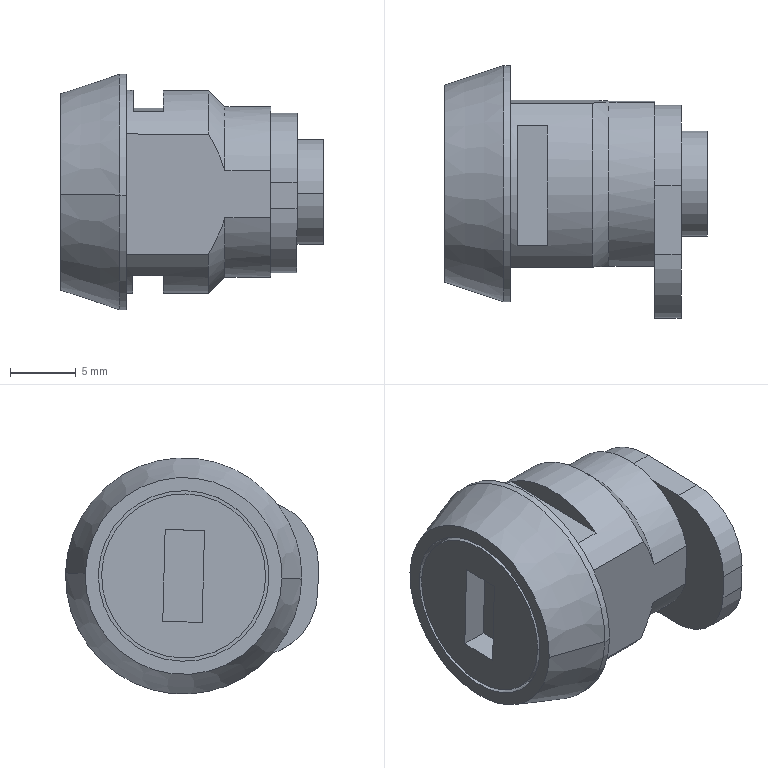Part | SolidWorks | features BaseBody 1 | 1 solid | 43 faces | box 20.01 x 19.274 x 18 mm | volume 3137 mm3 | plane 24 | cylinder 15 | cone 4 | commonest cylinder face diameters 13 x4 8 x2 10 x2 12.5 x2 15.5 x2 18 x2
STEP:
#1=CARTESIAN_POINT('',(-253.585,-3.449,-66.884));
#2=VERTEX_POINT('',#1);
#3=CARTESIAN_POINT('',(-253.585,-11.447,-67.09));
#4=VERTEX_POINT('',#3);
#5=CARTESIAN_POINT('',(-253.585,-7.448,-66.987));
#6=DIRECTION('',(-1.,-0.00003864,0.0008339));
#7=DIRECTION('',(-0.0000171,0.9997,0.02582));
#8=AXIS2_PLACEMENT_3D('',#5,#6,#7);
#9=CIRCLE('',#8,4.);
#10=EDGE_CURVE('',#2,#4,#9,.T.);
#11=ORIENTED_EDGE('',*,*,#10,.T.);
#12=CARTESIAN_POINT('',(-255.585,-11.447,-67.089));
#13=VERTEX_POINT('',#12);
#14=CARTESIAN_POINT('',(-255.585,-11.447,-67.089));
#15=DIRECTION('',(1.,0.00003864,-0.0008339));
#16=VECTOR('',#15,1000.);
#17=LINE('',#14,#16);
#18=EDGE_CURVE('',#13,#4,#17,.T.);
#19=ORIENTED_EDGE('',*,*,#18,.F.);
#20=CARTESIAN_POINT('',(-255.585,-3.449,-66.882));
#21=VERTEX_POINT('',#20);
#22=CARTESIAN_POINT('',(-255.585,-7.448,-66.986));
#23=DIRECTION('',(1.,0.00003864,-0.0008339));
#24=DIRECTION('',(0.0000171,-0.9997,-0.02582));
#25=AXIS2_PLACEMENT_3D('',#22,#23,#24);
#26=CIRCLE('',#25,4.);
#27=EDGE_CURVE('',#13,#21,#26,.T.);
#28=ORIENTED_EDGE('',*,*,#27,.T.);
#29=CARTESIAN_POINT('',(-255.585,-3.449,-66.882));
#30=DIRECTION('',(1.,0.00003864,-0.0008339));
#31=VECTOR('',#30,1000.);
#32=LINE('',#29,#31);
#33=EDGE_CURVE('',#21,#2,#32,.T.);
#34=ORIENTED_EDGE('',*,*,#33,.T.);
#35=EDGE_LOOP('',(#11,#19,#28,#34));
#36=FACE_OUTER_BOUND('',#35,.T.);
#37=CARTESIAN_POINT('',(-253.585,-7.448,-66.987));
#38=DIRECTION('',(-1.,-0.00003864,0.0008339));
#39=DIRECTION('',(0.0000171,-0.9997,-0.02582));
#40=AXIS2_PLACEMENT_3D('',#37,#38,#39);
#41=CYLINDRICAL_SURFACE('',#40,4.);
#42=ADVANCED_FACE('',(#36),#41,.T.);
#43=ORIENTED_EDGE('',*,*,#33,.F.);
#44=CARTESIAN_POINT('',(-255.585,-7.448,-66.986));
#45=DIRECTION('',(1.,0.00003864,-0.0008339));
#46=DIRECTION('',(-0.0000171,0.9997,0.02582));
#47=AXIS2_PLACEMENT_3D('',#44,#45,#46);
#48=CIRCLE('',#47,4.);
#49=EDGE_CURVE('',#21,#13,#48,.T.);
#50=ORIENTED_EDGE('',*,*,#49,.T.);
#51=ORIENTED_EDGE('',*,*,#18,.T.);
#52=CARTESIAN_POINT('',(-253.585,-7.448,-66.987));
#53=DIRECTION('',(-1.,-0.00003864,0.0008339));
#54=DIRECTION('',(0.0000171,-0.9997,-0.02582));
#55=AXIS2_PLACEMENT_3D('',#52,#53,#54);
#56=CIRCLE('',#55,4.);
#57=EDGE_CURVE('',#4,#2,#56,.T.);
#58=ORIENTED_EDGE('',*,*,#57,.T.);
#59=EDGE_LOOP('',(#43,#50,#51,#58));
#60=FACE_OUTER_BOUND('',#59,.T.);
#61=CARTESIAN_POINT('',(-253.585,-7.448,-66.987));
#62=DIRECTION('',(-1.,-0.00003864,0.0008339));
#63=DIRECTION('',(0.0000171,-0.9997,-0.02582));
#64=AXIS2_PLACEMENT_3D('',#61,#62,#63);
#65=CYLINDRICAL_SURFACE('',#64,4.);
#66=ADVANCED_FACE('',(#60),#65,.T.);
#67=ORIENTED_EDGE('',*,*,#57,.F.);
#68=ORIENTED_EDGE('',*,*,#10,.F.);
#69=EDGE_LOOP('',(#67,#68));
#70=FACE_OUTER_BOUND('',#69,.T.);
#71=CARTESIAN_POINT('',(-253.585,-7.448,-66.987));
#72=DIRECTION('',(1.,0.00003864,-0.0008339));
#73=DIRECTION('',(0.,-0.9989,-0.04628));
#74=AXIS2_PLACEMENT_3D('',#71,#72,#73);
#75=PLANE('',#74);
#76=ADVANCED_FACE('',(#70),#75,.T.);
#77=ORIENTED_EDGE('',*,*,#49,.F.);
#78=ORIENTED_EDGE('',*,*,#27,.F.);
#79=EDGE_LOOP('',(#77,#78));
#80=FACE_BOUND('',#79,.T.);
#81=CARTESIAN_POINT('',(-255.584,-17.72,-66.251));
#82=VERTEX_POINT('',#81);
#83=CARTESIAN_POINT('',(-255.58,-12.851,-61.123));
#84=VERTEX_POINT('',#83);
#85=CARTESIAN_POINT('',(-255.584,-12.722,-66.121));
#86=DIRECTION('',(-1.,-0.00003864,0.0008339));
#87=DIRECTION('',(0.0000171,-0.9997,-0.02582));
#88=AXIS2_PLACEMENT_3D('',#85,#86,#87);
#89=CIRCLE('',#88,5.);
#90=EDGE_CURVE('',#82,#84,#89,.T.);
#91=ORIENTED_EDGE('',*,*,#90,.F.);
#92=CARTESIAN_POINT('',(-255.585,-17.669,-68.25));
#93=VERTEX_POINT('',#92);
#94=CARTESIAN_POINT('',(-255.584,-17.72,-66.251));
#95=DIRECTION('',(-0.0008346,0.02582,-0.9997));
#96=VECTOR('',#95,1000.);
#97=LINE('',#94,#96);
#98=EDGE_CURVE('',#82,#93,#97,.T.);
#99=ORIENTED_EDGE('',*,*,#98,.T.);
#100=CARTESIAN_POINT('',(-255.59,-12.541,-73.119));
#101=VERTEX_POINT('',#100);
#102=CARTESIAN_POINT('',(-255.585,-12.67,-68.121));
#103=DIRECTION('',(-1.,-0.00003864,0.0008339));
#104=DIRECTION('',(-0.0008346,0.02582,-0.9997));
#105=AXIS2_PLACEMENT_3D('',#102,#103,#104);
#106=CIRCLE('',#105,5.);
#107=EDGE_CURVE('',#101,#93,#106,.T.);
#108=ORIENTED_EDGE('',*,*,#107,.F.);
#109=CARTESIAN_POINT('',(-255.59,-7.293,-72.984));
#110=VERTEX_POINT('',#109);
#111=CARTESIAN_POINT('',(-255.59,-7.293,-72.984));
#112=DIRECTION('',(0.0000171,-0.9997,-0.02582));
#113=VECTOR('',#112,1000.);
#114=LINE('',#111,#113);
#115=EDGE_CURVE('',#110,#101,#114,.T.);
#116=ORIENTED_EDGE('',*,*,#115,.F.);
#117=CARTESIAN_POINT('',(-255.58,-7.603,-60.988));
#118=VERTEX_POINT('',#117);
#119=CARTESIAN_POINT('',(-255.585,-7.448,-66.986));
#120=DIRECTION('',(-1.,-0.00003864,0.0008339));
#121=DIRECTION('',(-0.0000171,0.9997,0.02582));
#122=AXIS2_PLACEMENT_3D('',#119,#120,#121);
#123=CIRCLE('',#122,6.);
#124=EDGE_CURVE('',#118,#110,#123,.T.);
#125=ORIENTED_EDGE('',*,*,#124,.F.);
#126=CARTESIAN_POINT('',(-255.58,-12.851,-61.123));
#127=DIRECTION('',(-0.0000171,0.9997,0.02582));
#128=VECTOR('',#127,1000.);
#129=LINE('',#126,#128);
#130=EDGE_CURVE('',#84,#118,#129,.T.);
#131=ORIENTED_EDGE('',*,*,#130,.F.);
#132=EDGE_LOOP('',(#91,#99,#108,#116,#125,#131));
#133=FACE_OUTER_BOUND('',#132,.T.);
#134=CARTESIAN_POINT('',(-255.581,-20.047,-63.31));
#135=DIRECTION('',(1.,0.00003864,-0.0008339));
#136=DIRECTION('',(0.,-0.9989,-0.04628));
#137=AXIS2_PLACEMENT_3D('',#134,#135,#136);
#138=PLANE('',#137);
#139=ADVANCED_FACE('',(#80,#133),#138,.T.);
#140=CARTESIAN_POINT('',(-257.58,-12.851,-61.121));
#141=VERTEX_POINT('',#140);
#142=CARTESIAN_POINT('',(-257.58,-12.851,-61.121));
#143=DIRECTION('',(1.,0.00003864,-0.0008339));
#144=VECTOR('',#143,1000.);
#145=LINE('',#142,#144);
#146=EDGE_CURVE('',#141,#84,#145,.T.);
#147=ORIENTED_EDGE('',*,*,#146,.T.);
#148=ORIENTED_EDGE('',*,*,#130,.T.);
#149=CARTESIAN_POINT('',(-257.58,-7.603,-60.986));
#150=VERTEX_POINT('',#149);
#151=CARTESIAN_POINT('',(-255.58,-7.603,-60.988));
#152=DIRECTION('',(-1.,-0.00003864,0.0008339));
#153=VECTOR('',#152,1000.);
#154=LINE('',#151,#153);
#155=EDGE_CURVE('',#118,#150,#154,.T.);
#156=ORIENTED_EDGE('',*,*,#155,.T.);
#157=CARTESIAN_POINT('',(-257.58,-10.102,-61.05));
#158=VERTEX_POINT('',#157);
#159=CARTESIAN_POINT('',(-257.58,-10.102,-61.05));
#160=DIRECTION('',(-0.0000171,0.9997,0.02582));
#161=VECTOR('',#160,1000.);
#162=LINE('',#159,#161);
#163=EDGE_CURVE('',#158,#150,#162,.T.);
#164=ORIENTED_EDGE('',*,*,#163,.F.);
#165=CARTESIAN_POINT('',(-257.58,-12.851,-61.121));
#166=DIRECTION('',(-0.0000171,0.9997,0.02582));
#167=VECTOR('',#166,1000.);
#168=LINE('',#165,#167);
#169=EDGE_CURVE('',#141,#158,#168,.T.);
#170=ORIENTED_EDGE('',*,*,#169,.F.);
#171=EDGE_LOOP('',(#147,#148,#156,#164,#170));
#172=FACE_OUTER_BOUND('',#171,.T.);
#173=CARTESIAN_POINT('',(-255.58,-7.603,-60.988));
#174=DIRECTION('',(-0.0008346,0.02582,-0.9997));
#175=DIRECTION('',(-1.,0.,0.0008349));
#176=AXIS2_PLACEMENT_3D('',#173,#174,#175);
#177=PLANE('',#176);
#178=ADVANCED_FACE('',(#172),#177,.F.);
#179=CARTESIAN_POINT('',(-257.584,-17.72,-66.249));
#180=VERTEX_POINT('',#179);
#181=CARTESIAN_POINT('',(-257.584,-12.722,-66.12));
#182=DIRECTION('',(1.,0.00003864,-0.0008339));
#183=DIRECTION('',(0.0008346,-0.02582,0.9997));
#184=AXIS2_PLACEMENT_3D('',#181,#182,#183);
#185=CIRCLE('',#184,5.);
#186=EDGE_CURVE('',#141,#180,#185,.T.);
#187=ORIENTED_EDGE('',*,*,#186,.F.);
#188=ORIENTED_EDGE('',*,*,#169,.T.);
#189=CARTESIAN_POINT('',(-257.583,-13.742,-65.36));
#190=VERTEX_POINT('',#189);
#191=CARTESIAN_POINT('',(-257.585,-7.448,-66.984));
#192=DIRECTION('',(-1.,-0.00003864,0.0008339));
#193=DIRECTION('',(0.0002457,-0.9683,0.2498));
#194=AXIS2_PLACEMENT_3D('',#191,#192,#193);
#195=CIRCLE('',#194,6.5);
#196=EDGE_CURVE('',#190,#158,#195,.T.);
#197=ORIENTED_EDGE('',*,*,#196,.F.);
#198=CARTESIAN_POINT('',(-257.586,-13.65,-68.93));
#199=VERTEX_POINT('',#198);
#200=CARTESIAN_POINT('',(-257.583,-13.742,-65.36));
#201=DIRECTION('',(-0.0008346,0.02582,-0.9997));
#202=VECTOR('',#201,1000.);
#203=LINE('',#200,#202);
#204=EDGE_CURVE('',#190,#199,#203,.T.);
#205=ORIENTED_EDGE('',*,*,#204,.T.);
#206=CARTESIAN_POINT('',(-257.59,-9.792,-73.046));
#207=VERTEX_POINT('',#206);
#208=CARTESIAN_POINT('',(-257.585,-7.448,-66.984));
#209=DIRECTION('',(-1.,-0.00003864,0.0008339));
#210=DIRECTION('',(-0.0007639,-0.3607,-0.9327));
#211=AXIS2_PLACEMENT_3D('',#208,#209,#210);
#212=CIRCLE('',#211,6.5);
#213=EDGE_CURVE('',#207,#199,#212,.T.);
#214=ORIENTED_EDGE('',*,*,#213,.F.);
#215=CARTESIAN_POINT('',(-257.59,-12.541,-73.117));
#216=VERTEX_POINT('',#215);
#217=CARTESIAN_POINT('',(-257.59,-9.792,-73.046));
#218=DIRECTION('',(0.0000171,-0.9997,-0.02582));
#219=VECTOR('',#218,1000.);
#220=LINE('',#217,#219);
#221=EDGE_CURVE('',#207,#216,#220,.T.);
#222=ORIENTED_EDGE('',*,*,#221,.T.);
#223=CARTESIAN_POINT('',(-257.585,-17.669,-68.248));
#224=VERTEX_POINT('',#223);
#225=CARTESIAN_POINT('',(-257.585,-12.671,-68.119));
#226=DIRECTION('',(1.,0.00003864,-0.0008339));
#227=DIRECTION('',(0.0000171,-0.9997,-0.02582));
#228=AXIS2_PLACEMENT_3D('',#225,#226,#227);
#229=CIRCLE('',#228,5.);
#230=EDGE_CURVE('',#224,#216,#229,.T.);
#231=ORIENTED_EDGE('',*,*,#230,.F.);
#232=CARTESIAN_POINT('',(-257.585,-17.669,-68.248));
#233=DIRECTION('',(0.0008346,-0.02582,0.9997));
#234=VECTOR('',#233,1000.);
#235=LINE('',#232,#234);
#236=EDGE_CURVE('',#224,#180,#235,.T.);
#237=ORIENTED_EDGE('',*,*,#236,.T.);
#238=EDGE_LOOP('',(#187,#188,#197,#205,#214,#222,#231,#237));
#239=FACE_OUTER_BOUND('',#238,.T.);
#240=CARTESIAN_POINT('',(-257.581,-20.047,-63.308));
#241=DIRECTION('',(1.,0.00003864,-0.0008339));
#242=DIRECTION('',(0.,-0.9989,-0.04628));
#243=AXIS2_PLACEMENT_3D('',#240,#241,#242);
#244=PLANE('',#243);
#245=ADVANCED_FACE('',(#239),#244,.F.);
#246=CARTESIAN_POINT('',(-255.584,-17.72,-66.251));
#247=DIRECTION('',(-1.,-0.00003864,0.0008339));
#248=VECTOR('',#247,1000.);
#249=LINE('',#246,#248);
#250=EDGE_CURVE('',#82,#180,#249,.T.);
#251=ORIENTED_EDGE('',*,*,#250,.T.);
#252=ORIENTED_EDGE('',*,*,#236,.F.);
#253=CARTESIAN_POINT('',(-257.585,-17.669,-68.248));
#254=DIRECTION('',(1.,0.00003864,-0.0008339));
#255=VECTOR('',#254,1000.);
#256=LINE('',#253,#255);
#257=EDGE_CURVE('',#224,#93,#256,.T.);
#258=ORIENTED_EDGE('',*,*,#257,.T.);
#259=ORIENTED_EDGE('',*,*,#98,.F.);
#260=EDGE_LOOP('',(#251,#252,#258,#259));
#261=FACE_OUTER_BOUND('',#260,.T.);
#262=CARTESIAN_POINT('',(-247.578,-17.884,-59.908));
#263=DIRECTION('',(-0.0000171,0.9997,0.02582));
#264=DIRECTION('',(1.,0.,0.0006623));
#265=AXIS2_PLACEMENT_3D('',#262,#263,#264);
#266=PLANE('',#265);
#267=ADVANCED_FACE('',(#261),#266,.F.);
#268=ORIENTED_EDGE('',*,*,#257,.F.);
#269=ORIENTED_EDGE('',*,*,#230,.T.);
#270=CARTESIAN_POINT('',(-255.59,-12.541,-73.119));
#271=DIRECTION('',(-1.,-0.00003864,0.0008339));
#272=VECTOR('',#271,1000.);
#273=LINE('',#270,#272);
#274=EDGE_CURVE('',#101,#216,#273,.T.);
#275=ORIENTED_EDGE('',*,*,#274,.F.);
#276=ORIENTED_EDGE('',*,*,#107,.T.);
#277=EDGE_LOOP('',(#268,#269,#275,#276));
#278=FACE_OUTER_BOUND('',#277,.T.);
#279=CARTESIAN_POINT('',(-255.585,-12.67,-68.121));
#280=DIRECTION('',(-1.,-0.00003864,0.0008339));
#281=DIRECTION('',(0.0000171,-0.9997,-0.02582));
#282=AXIS2_PLACEMENT_3D('',#279,#280,#281);
#283=CYLINDRICAL_SURFACE('',#282,5.);
#284=ADVANCED_FACE('',(#278),#283,.T.);
#285=ORIENTED_EDGE('',*,*,#274,.T.);
#286=ORIENTED_EDGE('',*,*,#221,.F.);
#287=CARTESIAN_POINT('',(-257.59,-7.293,-72.982));
#288=VERTEX_POINT('',#287);
#289=CARTESIAN_POINT('',(-257.59,-7.293,-72.982));
#290=DIRECTION('',(0.0000171,-0.9997,-0.02582));
#291=VECTOR('',#290,1000.);
#292=LINE('',#289,#291);
#293=EDGE_CURVE('',#288,#207,#292,.T.);
#294=ORIENTED_EDGE('',*,*,#293,.F.);
#295=CARTESIAN_POINT('',(-257.59,-7.293,-72.982));
#296=DIRECTION('',(1.,0.00003864,-0.0008339));
#297=VECTOR('',#296,1000.);
#298=LINE('',#295,#297);
#299=EDGE_CURVE('',#288,#110,#298,.T.);
#300=ORIENTED_EDGE('',*,*,#299,.T.);
#301=ORIENTED_EDGE('',*,*,#115,.T.);
#302=EDGE_LOOP('',(#285,#286,#294,#300,#301));
#303=FACE_OUTER_BOUND('',#302,.T.);
#304=CARTESIAN_POINT('',(-255.59,-19.789,-73.306));
#305=DIRECTION('',(0.0008346,-0.02582,0.9997));
#306=DIRECTION('',(-0.9995,-0.03231,0.));
#307=AXIS2_PLACEMENT_3D('',#304,#305,#306);
#308=PLANE('',#307);
#309=ADVANCED_FACE('',(#303),#308,.F.);
#310=ORIENTED_EDGE('',*,*,#155,.F.);
#311=ORIENTED_EDGE('',*,*,#124,.T.);
#312=ORIENTED_EDGE('',*,*,#299,.F.);
#313=CARTESIAN_POINT('',(-257.585,-7.448,-66.984));
#314=DIRECTION('',(1.,0.00003864,-0.0008339));
#315=DIRECTION('',(-0.0008346,0.02582,-0.9997));
#316=AXIS2_PLACEMENT_3D('',#313,#314,#315);
#317=CIRCLE('',#316,6.);
#318=EDGE_CURVE('',#288,#150,#317,.T.);
#319=ORIENTED_EDGE('',*,*,#318,.T.);
#320=EDGE_LOOP('',(#310,#311,#312,#319));
#321=FACE_OUTER_BOUND('',#320,.T.);
#322=CARTESIAN_POINT('',(-255.585,-7.448,-66.986));
#323=DIRECTION('',(-1.,-0.00003864,0.0008339));
#324=DIRECTION('',(0.0000171,-0.9997,-0.02582));
#325=AXIS2_PLACEMENT_3D('',#322,#323,#324);
#326=CYLINDRICAL_SURFACE('',#325,6.);
#327=ADVANCED_FACE('',(#321),#326,.T.);
#328=ORIENTED_EDGE('',*,*,#163,.T.);
#329=ORIENTED_EDGE('',*,*,#318,.F.);
#330=ORIENTED_EDGE('',*,*,#293,.T.);
#331=CARTESIAN_POINT('',(-257.586,-1.154,-68.607));
#332=VERTEX_POINT('',#331);
#333=CARTESIAN_POINT('',(-257.585,-7.448,-66.984));
#334=DIRECTION('',(-1.,-0.00003864,0.0008339));
#335=DIRECTION('',(-0.0002457,0.9683,-0.2498));
#336=AXIS2_PLACEMENT_3D('',#333,#334,#335);
#337=CIRCLE('',#336,6.5);
#338=EDGE_CURVE('',#332,#207,#337,.T.);
#339=ORIENTED_EDGE('',*,*,#338,.F.);
#340=CARTESIAN_POINT('',(-257.583,-1.246,-65.038));
#341=VERTEX_POINT('',#340);
#342=CARTESIAN_POINT('',(-257.586,-1.154,-68.607));
#343=DIRECTION('',(0.0008346,-0.02582,0.9997));
#344=VECTOR('',#343,1000.);
#345=LINE('',#342,#344);
#346=EDGE_CURVE('',#332,#341,#345,.T.);
#347=ORIENTED_EDGE('',*,*,#346,.T.);
#348=CARTESIAN_POINT('',(-257.585,-7.448,-66.984));
#349=DIRECTION('',(-1.,-0.00003864,0.0008339));
#350=DIRECTION('',(0.000777,-0.4083,0.9128));
#351=AXIS2_PLACEMENT_3D('',#348,#349,#350);
#352=CIRCLE('',#351,6.5);
#353=EDGE_CURVE('',#158,#341,#352,.T.);
#354=ORIENTED_EDGE('',*,*,#353,.F.);
#355=EDGE_LOOP('',(#328,#329,#330,#339,#347,#354));
#356=FACE_OUTER_BOUND('',#355,.T.);
#357=CARTESIAN_POINT('',(-257.585,-7.448,-66.984));
#358=DIRECTION('',(1.,0.00003864,-0.0008339));
#359=DIRECTION('',(0.,-0.9989,-0.04628));
#360=AXIS2_PLACEMENT_3D('',#357,#358,#359);
#361=PLANE('',#360);
#362=ADVANCED_FACE('',(#356),#361,.T.);
#363=CARTESIAN_POINT('',(-261.083,-1.246,-65.035));
#364=VERTEX_POINT('',#363);
#365=CARTESIAN_POINT('',(-261.083,-13.742,-65.358));
#366=VERTEX_POINT('',#365);
#367=CARTESIAN_POINT('',(-261.085,-7.448,-66.981));
#368=DIRECTION('',(1.,0.00003864,-0.0008339));
#369=DIRECTION('',(0.0002128,0.9541,0.2994));
#370=AXIS2_PLACEMENT_3D('',#367,#368,#369);
#371=CIRCLE('',#370,6.5);
#372=EDGE_CURVE('',#364,#366,#371,.T.);
#373=ORIENTED_EDGE('',*,*,#372,.T.);
#374=CARTESIAN_POINT('',(-257.583,-13.742,-65.36));
#375=DIRECTION('',(-1.,-0.00003864,0.0008339));
#376=VECTOR('',#375,1000.);
#377=LINE('',#374,#376);
#378=EDGE_CURVE('',#190,#366,#377,.T.);
#379=ORIENTED_EDGE('',*,*,#378,.F.);
#380=ORIENTED_EDGE('',*,*,#196,.T.);
#381=ORIENTED_EDGE('',*,*,#353,.T.);
#382=CARTESIAN_POINT('',(-261.083,-1.246,-65.035));
#383=DIRECTION('',(1.,0.00003864,-0.0008339));
#384=VECTOR('',#383,1000.);
#385=LINE('',#382,#384);
#386=EDGE_CURVE('',#364,#341,#385,.T.);
#387=ORIENTED_EDGE('',*,*,#386,.F.);
#388=EDGE_LOOP('',(#373,#379,#380,#381,#387));
#389=FACE_OUTER_BOUND('',#388,.T.);
#390=CARTESIAN_POINT('',(-262.585,-7.448,-66.98));
#391=DIRECTION('',(1.,0.00003864,-0.0008339));
#392=DIRECTION('',(-0.0000171,0.9997,0.02582));
#393=AXIS2_PLACEMENT_3D('',#390,#391,#392);
#394=CYLINDRICAL_SURFACE('',#393,6.5);
#395=ADVANCED_FACE('',(#389),#394,.T.);
#396=CARTESIAN_POINT('',(-268.581,-1.319,-62.232));
#397=VERTEX_POINT('',#396);
#398=CARTESIAN_POINT('',(-262.331,-1.319,-62.238));
#399=VERTEX_POINT('',#398);
#400=CARTESIAN_POINT('',(-268.581,-1.319,-62.232));
#401=DIRECTION('',(1.,0.00003864,-0.0008339));
#402=VECTOR('',#401,1000.);
#403=LINE('',#400,#402);
#404=EDGE_CURVE('',#397,#399,#403,.T.);
#405=ORIENTED_EDGE('',*,*,#404,.T.);
#406=CARTESIAN_POINT('',(-262.331,-1.319,-62.238));
#407=CARTESIAN_POINT('',(-262.029,-1.305,-62.75));
#408=CARTESIAN_POINT('',(-261.774,-1.293,-63.238));
#409=CARTESIAN_POINT('',(-261.363,-1.269,-64.16));
#410=CARTESIAN_POINT('',(-261.201,-1.257,-64.606));
#411=CARTESIAN_POINT('',(-261.083,-1.246,-65.035));
#412=B_SPLINE_CURVE_WITH_KNOTS('',3,(#406,#407,#408,#409,#410,#411),.UNSPECIFIED.,.F.,.F.,(4,2,4),(0.,0.5,1.),.UNSPECIFIED.);
#413=EDGE_CURVE('',#399,#364,#412,.T.);
#414=ORIENTED_EDGE('',*,*,#413,.T.);
#415=ORIENTED_EDGE('',*,*,#386,.T.);
#416=ORIENTED_EDGE('',*,*,#346,.F.);
#417=CARTESIAN_POINT('',(-261.086,-1.154,-68.604));
#418=VERTEX_POINT('',#417);
#419=CARTESIAN_POINT('',(-257.586,-1.154,-68.607));
#420=DIRECTION('',(-1.,-0.00003864,0.0008339));
#421=VECTOR('',#420,1000.);
#422=LINE('',#419,#421);
#423=EDGE_CURVE('',#332,#418,#422,.T.);
#424=ORIENTED_EDGE('',*,*,#423,.T.);
#425=CARTESIAN_POINT('',(-262.339,-1.082,-71.4));
#426=VERTEX_POINT('',#425);
#427=CARTESIAN_POINT('',(-261.086,-1.154,-68.604));
#428=CARTESIAN_POINT('',(-261.146,-1.149,-68.822));
#429=CARTESIAN_POINT('',(-261.253,-1.14,-69.154));
#430=CARTESIAN_POINT('',(-261.408,-1.13,-69.553));
#431=CARTESIAN_POINT('',(-261.481,-1.125,-69.727));
#432=CARTESIAN_POINT('',(-261.531,-1.122,-69.843));
#433=CARTESIAN_POINT('',(-261.557,-1.121,-69.903));
#434=CARTESIAN_POINT('',(-261.788,-1.107,-70.415));
#435=CARTESIAN_POINT('',(-262.04,-1.095,-70.895));
#436=CARTESIAN_POINT('',(-262.339,-1.082,-71.4));
#437=B_SPLINE_CURVE_WITH_KNOTS('',3,(#427,#428,#429,#430,#431,#432,#433,#434,#435,#436),.UNSPECIFIED.,.F.,.F.,(4,1,1,2,2,4),(0.,0.25,0.375,0.4375,0.5,1.),.UNSPECIFIED.);
#438=EDGE_CURVE('',#418,#426,#437,.T.);
#439=ORIENTED_EDGE('',*,*,#438,.T.);
#440=CARTESIAN_POINT('',(-268.589,-1.082,-71.394));
#441=VERTEX_POINT('',#440);
#442=CARTESIAN_POINT('',(-262.339,-1.082,-71.4));
#443=DIRECTION('',(-1.,-0.00003864,0.0008339));
#444=VECTOR('',#443,1000.);
#445=LINE('',#442,#444);
#446=EDGE_CURVE('',#426,#441,#445,.T.);
#447=ORIENTED_EDGE('',*,*,#446,.T.);
#448=CARTESIAN_POINT('',(-268.589,-1.082,-71.394));
#449=DIRECTION('',(0.0008346,-0.02582,0.9997));
#450=VECTOR('',#449,1000.);
#451=LINE('',#448,#450);
#452=EDGE_CURVE('',#441,#397,#451,.T.);
#453=ORIENTED_EDGE('',*,*,#452,.T.);
#454=EDGE_LOOP('',(#405,#414,#415,#416,#424,#439,#447,#453));
#455=FACE_OUTER_BOUND('',#454,.T.);
#456=CARTESIAN_POINT('',(-296.984,-1.473,-56.266));
#457=DIRECTION('',(0.0000171,-0.9997,-0.02582));
#458=DIRECTION('',(0.,0.02582,-0.9997));
#459=AXIS2_PLACEMENT_3D('',#456,#457,#458);
#460=PLANE('',#459);
#461=ADVANCED_FACE('',(#455),#460,.F.);
#462=ORIENTED_EDGE('',*,*,#452,.F.);
#463=CARTESIAN_POINT('',(-268.588,-13.578,-71.717));
#464=VERTEX_POINT('',#463);
#465=CARTESIAN_POINT('',(-268.585,-7.449,-66.975));
#466=DIRECTION('',(1.,0.00003864,-0.0008339));
#467=DIRECTION('',(-0.0004797,-0.7909,-0.6119));
#468=AXIS2_PLACEMENT_3D('',#465,#466,#467);
#469=CIRCLE('',#468,7.75);
#470=EDGE_CURVE('',#464,#441,#469,.T.);
#471=ORIENTED_EDGE('',*,*,#470,.F.);
#472=CARTESIAN_POINT('',(-268.581,-13.815,-62.555));
#473=VERTEX_POINT('',#472);
#474=CARTESIAN_POINT('',(-268.581,-13.815,-62.555));
#475=DIRECTION('',(-0.0008346,0.02582,-0.9997));
#476=VECTOR('',#475,1000.);
#477=LINE('',#474,#476);
#478=EDGE_CURVE('',#473,#464,#477,.T.);
#479=ORIENTED_EDGE('',*,*,#478,.F.);
#480=CARTESIAN_POINT('',(-268.585,-7.449,-66.975));
#481=DIRECTION('',(1.,0.00003864,-0.0008339));
#482=DIRECTION('',(0.0004797,0.7909,0.6119));
#483=AXIS2_PLACEMENT_3D('',#480,#481,#482);
#484=CIRCLE('',#483,7.75);
#485=EDGE_CURVE('',#397,#473,#484,.T.);
#486=ORIENTED_EDGE('',*,*,#485,.F.);
#487=EDGE_LOOP('',(#462,#471,#479,#486));
#488=FACE_BOUND('',#487,.T.);
#489=CARTESIAN_POINT('',(-268.585,-16.446,-67.207));
#490=VERTEX_POINT('',#489);
#491=CARTESIAN_POINT('',(-268.585,1.548,-66.742));
#492=VERTEX_POINT('',#491);
#493=CARTESIAN_POINT('',(-268.585,-7.449,-66.975));
#494=DIRECTION('',(-1.,-0.00003864,0.0008339));
#495=DIRECTION('',(0.0000171,-0.9997,-0.02582));
#496=AXIS2_PLACEMENT_3D('',#493,#494,#495);
#497=CIRCLE('',#496,9.);
#498=EDGE_CURVE('',#490,#492,#497,.T.);
#499=ORIENTED_EDGE('',*,*,#498,.F.);
#500=CARTESIAN_POINT('',(-268.585,-7.449,-66.975));
#501=DIRECTION('',(-1.,-0.00003864,0.0008339));
#502=DIRECTION('',(-0.0000171,0.9997,0.02582));
#503=AXIS2_PLACEMENT_3D('',#500,#501,#502);
#504=CIRCLE('',#503,9.);
#505=EDGE_CURVE('',#492,#490,#504,.T.);
#506=ORIENTED_EDGE('',*,*,#505,.F.);
#507=EDGE_LOOP('',(#499,#506));
#508=FACE_OUTER_BOUND('',#507,.T.);
#509=CARTESIAN_POINT('',(-268.585,-7.449,-66.975));
#510=DIRECTION('',(-1.,-0.00003864,0.0008339));
#511=DIRECTION('',(-0.00003864,1.,0.));
#512=AXIS2_PLACEMENT_3D('',#509,#510,#511);
#513=PLANE('',#512);
#514=ADVANCED_FACE('',(#488,#508),#513,.F.);
#515=CARTESIAN_POINT('',(-269.085,-16.446,-67.207));
#516=VERTEX_POINT('',#515);
#517=CARTESIAN_POINT('',(-269.085,1.548,-66.742));
#518=VERTEX_POINT('',#517);
#519=CARTESIAN_POINT('',(-269.085,-7.449,-66.974));
#520=DIRECTION('',(1.,0.00003864,-0.0008339));
#521=DIRECTION('',(0.0000171,-0.9997,-0.02582));
#522=AXIS2_PLACEMENT_3D('',#519,#520,#521);
#523=CIRCLE('',#522,9.);
#524=EDGE_CURVE('',#516,#518,#523,.T.);
#525=ORIENTED_EDGE('',*,*,#524,.T.);
#526=CARTESIAN_POINT('',(-268.585,1.548,-66.742));
#527=DIRECTION('',(-1.,-0.00003864,0.0008339));
#528=VECTOR('',#527,1000.);
#529=LINE('',#526,#528);
#530=EDGE_CURVE('',#492,#518,#529,.T.);
#531=ORIENTED_EDGE('',*,*,#530,.F.);
#532=ORIENTED_EDGE('',*,*,#505,.T.);
#533=CARTESIAN_POINT('',(-268.585,-16.446,-67.207));
#534=DIRECTION('',(-1.,-0.00003864,0.0008339));
#535=VECTOR('',#534,1000.);
#536=LINE('',#533,#535);
#537=EDGE_CURVE('',#490,#516,#536,.T.);
#538=ORIENTED_EDGE('',*,*,#537,.T.);
#539=EDGE_LOOP('',(#525,#531,#532,#538));
#540=FACE_OUTER_BOUND('',#539,.T.);
#541=CARTESIAN_POINT('',(-273.585,-7.449,-66.971));
#542=DIRECTION('',(1.,0.00003864,-0.0008339));
#543=DIRECTION('',(-0.0000171,0.9997,0.02582));
#544=AXIS2_PLACEMENT_3D('',#541,#542,#543);
#545=CYLINDRICAL_SURFACE('',#544,9.);
#546=ADVANCED_FACE('',(#540),#545,.T.);
#547=ORIENTED_EDGE('',*,*,#537,.F.);
#548=ORIENTED_EDGE('',*,*,#498,.T.);
#549=ORIENTED_EDGE('',*,*,#530,.T.);
#550=CARTESIAN_POINT('',(-269.085,-7.449,-66.974));
#551=DIRECTION('',(1.,0.00003864,-0.0008339));
#552=DIRECTION('',(-0.0000171,0.9997,0.02582));
#553=AXIS2_PLACEMENT_3D('',#550,#551,#552);
#554=CIRCLE('',#553,9.);
#555=EDGE_CURVE('',#518,#516,#554,.T.);
#556=ORIENTED_EDGE('',*,*,#555,.T.);
#557=EDGE_LOOP('',(#547,#548,#549,#556));
#558=FACE_OUTER_BOUND('',#557,.T.);
#559=CARTESIAN_POINT('',(-273.585,-7.449,-66.971));
#560=DIRECTION('',(1.,0.00003864,-0.0008339));
#561=DIRECTION('',(-0.0000171,0.9997,0.02582));
#562=AXIS2_PLACEMENT_3D('',#559,#560,#561);
#563=CYLINDRICAL_SURFACE('',#562,9.);
#564=ADVANCED_FACE('',(#558),#563,.T.);
#565=CARTESIAN_POINT('',(-273.585,-14.946,-67.164));
#566=VERTEX_POINT('',#565);
#567=CARTESIAN_POINT('',(-269.085,-16.446,-67.207));
#568=DIRECTION('',(-0.9487,0.3161,0.008955));
#569=VECTOR('',#568,1000.);
#570=LINE('',#567,#569);
#571=EDGE_CURVE('',#516,#566,#570,.T.);
#572=ORIENTED_EDGE('',*,*,#571,.F.);
#573=ORIENTED_EDGE('',*,*,#555,.F.);
#574=CARTESIAN_POINT('',(-273.585,0.04878,-66.777));
#575=VERTEX_POINT('',#574);
#576=CARTESIAN_POINT('',(-269.085,1.548,-66.742));
#577=DIRECTION('',(-0.9487,-0.3162,-0.007373));
#578=VECTOR('',#577,1000.);
#579=LINE('',#576,#578);
#580=EDGE_CURVE('',#518,#575,#579,.T.);
#581=ORIENTED_EDGE('',*,*,#580,.T.);
#582=CARTESIAN_POINT('',(-273.585,-7.449,-66.971));
#583=DIRECTION('',(1.,0.00003864,-0.0008339));
#584=DIRECTION('',(-0.0000171,0.9997,0.02582));
#585=AXIS2_PLACEMENT_3D('',#582,#583,#584);
#586=CIRCLE('',#585,7.5);
#587=EDGE_CURVE('',#575,#566,#586,.T.);
#588=ORIENTED_EDGE('',*,*,#587,.T.);
#589=EDGE_LOOP('',(#572,#573,#581,#588));
#590=FACE_OUTER_BOUND('',#589,.T.);
#591=CARTESIAN_POINT('',(-271.335,-7.449,-66.972));
#592=DIRECTION('',(1.,0.00003864,-0.0008339));
#593=DIRECTION('',(-0.0000171,0.9997,0.02582));
#594=AXIS2_PLACEMENT_3D('',#591,#592,#593);
#595=CONICAL_SURFACE('',#594,8.25,0.3218);
#596=ADVANCED_FACE('',(#590),#595,.T.);
#597=CARTESIAN_POINT('',(-273.585,-0.9509,-66.803));
#598=VERTEX_POINT('',#597);
#599=CARTESIAN_POINT('',(-273.585,-13.947,-67.138));
#600=VERTEX_POINT('',#599);
#601=CARTESIAN_POINT('',(-273.585,-7.449,-66.971));
#602=DIRECTION('',(-1.,-0.00003864,0.0008339));
#603=DIRECTION('',(-0.0000171,0.9997,0.02582));
#604=AXIS2_PLACEMENT_3D('',#601,#602,#603);
#605=CIRCLE('',#604,6.5);
#606=EDGE_CURVE('',#598,#600,#605,.T.);
#607=ORIENTED_EDGE('',*,*,#606,.F.);
#608=CARTESIAN_POINT('',(-273.585,-7.449,-66.971));
#609=DIRECTION('',(-1.,-0.00003864,0.0008339));
#610=DIRECTION('',(0.0000171,-0.9997,-0.02582));
#611=AXIS2_PLACEMENT_3D('',#608,#609,#610);
#612=CIRCLE('',#611,6.5);
#613=EDGE_CURVE('',#600,#598,#612,.T.);
#614=ORIENTED_EDGE('',*,*,#613,.F.);
#615=EDGE_LOOP('',(#607,#614));
#616=FACE_BOUND('',#615,.T.);
#617=ORIENTED_EDGE('',*,*,#587,.F.);
#618=CARTESIAN_POINT('',(-273.585,-7.449,-66.971));
#619=DIRECTION('',(1.,0.00003864,-0.0008339));
#620=DIRECTION('',(0.0000171,-0.9997,-0.02582));
#621=AXIS2_PLACEMENT_3D('',#618,#619,#620);
#622=CIRCLE('',#621,7.5);
#623=EDGE_CURVE('',#566,#575,#622,.T.);
#624=ORIENTED_EDGE('',*,*,#623,.F.);
#625=EDGE_LOOP('',(#617,#624));
#626=FACE_OUTER_BOUND('',#625,.T.);
#627=CARTESIAN_POINT('',(-273.585,-7.449,-66.971));
#628=DIRECTION('',(-1.,-0.00003864,0.0008339));
#629=DIRECTION('',(-0.00003864,1.,0.));
#630=AXIS2_PLACEMENT_3D('',#627,#628,#629);
#631=PLANE('',#630);
#632=ADVANCED_FACE('',(#616,#626),#631,.T.);
#633=ORIENTED_EDGE('',*,*,#623,.T.);
#634=ORIENTED_EDGE('',*,*,#580,.F.);
#635=ORIENTED_EDGE('',*,*,#524,.F.);
#636=ORIENTED_EDGE('',*,*,#571,.T.);
#637=EDGE_LOOP('',(#633,#634,#635,#636));
#638=FACE_OUTER_BOUND('',#637,.T.);
#639=CARTESIAN_POINT('',(-271.335,-7.449,-66.972));
#640=DIRECTION('',(1.,0.00003864,-0.0008339));
#641=DIRECTION('',(-0.0000171,0.9997,0.02582));
#642=AXIS2_PLACEMENT_3D('',#639,#640,#641);
#643=CONICAL_SURFACE('',#642,8.25,0.3218);
#644=ADVANCED_FACE('',(#638),#643,.T.);
#645=CARTESIAN_POINT('',(-271.585,-0.9508,-66.804));
#646=VERTEX_POINT('',#645);
#647=CARTESIAN_POINT('',(-271.585,-13.946,-67.14));
#648=VERTEX_POINT('',#647);
#649=CARTESIAN_POINT('',(-271.585,-7.449,-66.972));
#650=DIRECTION('',(1.,0.00003864,-0.0008339));
#651=DIRECTION('',(-0.0000171,0.9997,0.02582));
#652=AXIS2_PLACEMENT_3D('',#649,#650,#651);
#653=CIRCLE('',#652,6.5);
#654=EDGE_CURVE('',#646,#648,#653,.T.);
#655=ORIENTED_EDGE('',*,*,#654,.T.);
#656=CARTESIAN_POINT('',(-273.585,-13.947,-67.138));
#657=DIRECTION('',(1.,0.00003864,-0.0008339));
#658=VECTOR('',#657,1000.);
#659=LINE('',#656,#658);
#660=EDGE_CURVE('',#600,#648,#659,.T.);
#661=ORIENTED_EDGE('',*,*,#660,.F.);
#662=ORIENTED_EDGE('',*,*,#613,.T.);
#663=CARTESIAN_POINT('',(-273.585,-0.9509,-66.803));
#664=DIRECTION('',(1.,0.00003864,-0.0008339));
#665=VECTOR('',#664,1000.);
#666=LINE('',#663,#665);
#667=EDGE_CURVE('',#598,#646,#666,.T.);
#668=ORIENTED_EDGE('',*,*,#667,.T.);
#669=EDGE_LOOP('',(#655,#661,#662,#668));
#670=FACE_OUTER_BOUND('',#669,.T.);
#671=CARTESIAN_POINT('',(-271.585,-7.449,-66.972));
#672=DIRECTION('',(-1.,-0.00003864,0.0008339));
#673=DIRECTION('',(0.0000171,-0.9997,-0.02582));
#674=AXIS2_PLACEMENT_3D('',#671,#672,#673);
#675=CYLINDRICAL_SURFACE('',#674,6.5);
#676=ADVANCED_FACE('',(#670),#675,.F.);
#677=ORIENTED_EDGE('',*,*,#667,.F.);
#678=ORIENTED_EDGE('',*,*,#606,.T.);
#679=ORIENTED_EDGE('',*,*,#660,.T.);
#680=CARTESIAN_POINT('',(-271.585,-7.449,-66.972));
#681=DIRECTION('',(1.,0.00003864,-0.0008339));
#682=DIRECTION('',(0.0000171,-0.9997,-0.02582));
#683=AXIS2_PLACEMENT_3D('',#680,#681,#682);
#684=CIRCLE('',#683,6.5);
#685=EDGE_CURVE('',#648,#646,#684,.T.);
#686=ORIENTED_EDGE('',*,*,#685,.T.);
#687=EDGE_LOOP('',(#677,#678,#679,#686));
#688=FACE_OUTER_BOUND('',#687,.T.);
#689=CARTESIAN_POINT('',(-271.585,-7.449,-66.972));
#690=DIRECTION('',(-1.,-0.00003864,0.0008339));
#691=DIRECTION('',(0.0000171,-0.9997,-0.02582));
#692=AXIS2_PLACEMENT_3D('',#689,#690,#691);
#693=CYLINDRICAL_SURFACE('',#692,6.5);
#694=ADVANCED_FACE('',(#688),#693,.F.);
#695=CARTESIAN_POINT('',(-271.585,-1.201,-66.811));
#696=VERTEX_POINT('',#695);
#697=CARTESIAN_POINT('',(-271.585,-13.697,-67.134));
#698=VERTEX_POINT('',#697);
#699=CARTESIAN_POINT('',(-271.585,-7.449,-66.972));
#700=DIRECTION('',(-1.,-0.00003864,0.0008339));
#701=DIRECTION('',(-0.0000171,0.9997,0.02582));
#702=AXIS2_PLACEMENT_3D('',#699,#700,#701);
#703=CIRCLE('',#702,6.25);
#704=EDGE_CURVE('',#696,#698,#703,.T.);
#705=ORIENTED_EDGE('',*,*,#704,.F.);
#706=CARTESIAN_POINT('',(-271.585,-7.449,-66.972));
#707=DIRECTION('',(-1.,-0.00003864,0.0008339));
#708=DIRECTION('',(0.0000171,-0.9997,-0.02582));
#709=AXIS2_PLACEMENT_3D('',#706,#707,#708);
#710=CIRCLE('',#709,6.25);
#711=EDGE_CURVE('',#698,#696,#710,.T.);
#712=ORIENTED_EDGE('',*,*,#711,.F.);
#713=EDGE_LOOP('',(#705,#712));
#714=FACE_BOUND('',#713,.T.);
#715=ORIENTED_EDGE('',*,*,#685,.F.);
#716=ORIENTED_EDGE('',*,*,#654,.F.);
#717=EDGE_LOOP('',(#715,#716));
#718=FACE_OUTER_BOUND('',#717,.T.);
#719=CARTESIAN_POINT('',(-271.585,-7.449,-66.972));
#720=DIRECTION('',(-1.,-0.00003864,0.0008339));
#721=DIRECTION('',(-0.00003864,1.,0.));
#722=AXIS2_PLACEMENT_3D('',#719,#720,#721);
#723=PLANE('',#722);
#724=ADVANCED_FACE('',(#714,#718),#723,.T.);
#725=CARTESIAN_POINT('',(-273.585,-1.201,-66.809));
#726=VERTEX_POINT('',#725);
#727=CARTESIAN_POINT('',(-273.585,-1.201,-66.809));
#728=DIRECTION('',(1.,0.00003864,-0.0008339));
#729=VECTOR('',#728,1000.);
#730=LINE('',#727,#729);
#731=EDGE_CURVE('',#726,#696,#730,.T.);
#732=ORIENTED_EDGE('',*,*,#731,.F.);
#733=CARTESIAN_POINT('',(-273.585,-13.697,-67.132));
#734=VERTEX_POINT('',#733);
#735=CARTESIAN_POINT('',(-273.585,-7.449,-66.971));
#736=DIRECTION('',(1.,0.00003864,-0.0008339));
#737=DIRECTION('',(-0.0000171,0.9997,0.02582));
#738=AXIS2_PLACEMENT_3D('',#735,#736,#737);
#739=CIRCLE('',#738,6.25);
#740=EDGE_CURVE('',#726,#734,#739,.T.);
#741=ORIENTED_EDGE('',*,*,#740,.T.);
#742=CARTESIAN_POINT('',(-273.585,-13.697,-67.132));
#743=DIRECTION('',(1.,0.00003864,-0.0008339));
#744=VECTOR('',#743,1000.);
#745=LINE('',#742,#744);
#746=EDGE_CURVE('',#734,#698,#745,.T.);
#747=ORIENTED_EDGE('',*,*,#746,.T.);
#748=ORIENTED_EDGE('',*,*,#711,.T.);
#749=EDGE_LOOP('',(#732,#741,#747,#748));
#750=FACE_OUTER_BOUND('',#749,.T.);
#751=CARTESIAN_POINT('',(-271.585,-7.449,-66.972));
#752=DIRECTION('',(-1.,-0.00003864,0.0008339));
#753=DIRECTION('',(0.0000171,-0.9997,-0.02582));
#754=AXIS2_PLACEMENT_3D('',#751,#752,#753);
#755=CYLINDRICAL_SURFACE('',#754,6.25);
#756=ADVANCED_FACE('',(#750),#755,.T.);
#757=ORIENTED_EDGE('',*,*,#704,.T.);
#758=ORIENTED_EDGE('',*,*,#746,.F.);
#759=CARTESIAN_POINT('',(-273.585,-7.449,-66.971));
#760=DIRECTION('',(1.,0.00003864,-0.0008339));
#761=DIRECTION('',(0.0000171,-0.9997,-0.02582));
#762=AXIS2_PLACEMENT_3D('',#759,#760,#761);
#763=CIRCLE('',#762,6.25);
#764=EDGE_CURVE('',#734,#726,#763,.T.);
#765=ORIENTED_EDGE('',*,*,#764,.T.);
#766=ORIENTED_EDGE('',*,*,#731,.T.);
#767=EDGE_LOOP('',(#757,#758,#765,#766));
#768=FACE_OUTER_BOUND('',#767,.T.);
#769=CARTESIAN_POINT('',(-271.585,-7.449,-66.972));
#770=DIRECTION('',(-1.,-0.00003864,0.0008339));
#771=DIRECTION('',(0.0000171,-0.9997,-0.02582));
#772=AXIS2_PLACEMENT_3D('',#769,#770,#771);
#773=CYLINDRICAL_SURFACE('',#772,6.25);
#774=ADVANCED_FACE('',(#768),#773,.T.);
#775=CARTESIAN_POINT('',(-273.582,-9.039,-63.51));
#776=VERTEX_POINT('',#775);
#777=CARTESIAN_POINT('',(-273.588,-8.858,-70.508));
#778=VERTEX_POINT('',#777);
#779=CARTESIAN_POINT('',(-273.582,-9.039,-63.51));
#780=DIRECTION('',(-0.0008346,0.02582,-0.9997));
#781=VECTOR('',#780,1000.);
#782=LINE('',#779,#781);
#783=EDGE_CURVE('',#776,#778,#782,.T.);
#784=ORIENTED_EDGE('',*,*,#783,.T.);
#785=CARTESIAN_POINT('',(-273.588,-5.859,-70.431));
#786=VERTEX_POINT('',#785);
#787=CARTESIAN_POINT('',(-273.588,-8.858,-70.508));
#788=DIRECTION('',(-0.0000171,0.9997,0.02582));
#789=VECTOR('',#788,1000.);
#790=LINE('',#787,#789);
#791=EDGE_CURVE('',#778,#786,#790,.T.);
#792=ORIENTED_EDGE('',*,*,#791,.T.);
#793=CARTESIAN_POINT('',(-273.582,-6.04,-63.433));
#794=VERTEX_POINT('',#793);
#795=CARTESIAN_POINT('',(-273.588,-5.859,-70.431));
#796=DIRECTION('',(0.0008346,-0.02582,0.9997));
#797=VECTOR('',#796,1000.);
#798=LINE('',#795,#797);
#799=EDGE_CURVE('',#786,#794,#798,.T.);
#800=ORIENTED_EDGE('',*,*,#799,.T.);
#801=CARTESIAN_POINT('',(-273.582,-6.04,-63.433));
#802=DIRECTION('',(0.0000171,-0.9997,-0.02582));
#803=VECTOR('',#802,1000.);
#804=LINE('',#801,#803);
#805=EDGE_CURVE('',#794,#776,#804,.T.);
#806=ORIENTED_EDGE('',*,*,#805,.T.);
#807=EDGE_LOOP('',(#784,#792,#800,#806));
#808=FACE_BOUND('',#807,.T.);
#809=ORIENTED_EDGE('',*,*,#764,.F.);
#810=ORIENTED_EDGE('',*,*,#740,.F.);
#811=EDGE_LOOP('',(#809,#810));
#812=FACE_OUTER_BOUND('',#811,.T.);
#813=CARTESIAN_POINT('',(-273.585,-7.449,-66.971));
#814=DIRECTION('',(-1.,-0.00003864,0.0008339));
#815=DIRECTION('',(-0.00003864,1.,0.));
#816=AXIS2_PLACEMENT_3D('',#813,#814,#815);
#817=PLANE('',#816);
#818=ADVANCED_FACE('',(#808,#812),#817,.T.);
#819=CARTESIAN_POINT('',(-271.582,-6.039,-63.435));
#820=VERTEX_POINT('',#819);
#821=CARTESIAN_POINT('',(-273.582,-6.04,-63.433));
#822=DIRECTION('',(1.,0.00003864,-0.0008339));
#823=VECTOR('',#822,1000.);
#824=LINE('',#821,#823);
#825=EDGE_CURVE('',#794,#820,#824,.T.);
#826=ORIENTED_EDGE('',*,*,#825,.T.);
#827=CARTESIAN_POINT('',(-271.582,-9.038,-63.512));
#828=VERTEX_POINT('',#827);
#829=CARTESIAN_POINT('',(-271.582,-6.039,-63.435));
#830=DIRECTION('',(0.0000171,-0.9997,-0.02582));
#831=VECTOR('',#830,1000.);
#832=LINE('',#829,#831);
#833=EDGE_CURVE('',#820,#828,#832,.T.);
#834=ORIENTED_EDGE('',*,*,#833,.T.);
#835=CARTESIAN_POINT('',(-273.582,-9.039,-63.51));
#836=DIRECTION('',(1.,0.00003864,-0.0008339));
#837=VECTOR('',#836,1000.);
#838=LINE('',#835,#837);
#839=EDGE_CURVE('',#776,#828,#838,.T.);
#840=ORIENTED_EDGE('',*,*,#839,.F.);
#841=ORIENTED_EDGE('',*,*,#805,.F.);
#842=EDGE_LOOP('',(#826,#834,#840,#841));
#843=FACE_OUTER_BOUND('',#842,.T.);
#844=CARTESIAN_POINT('',(-271.582,-9.038,-63.512));
#845=DIRECTION('',(0.0008346,-0.02582,0.9997));
#846=DIRECTION('',(-0.9995,-0.03231,0.));
#847=AXIS2_PLACEMENT_3D('',#844,#845,#846);
#848=PLANE('',#847);
#849=ADVANCED_FACE('',(#843),#848,.F.);
#850=ORIENTED_EDGE('',*,*,#839,.T.);
#851=CARTESIAN_POINT('',(-271.588,-8.858,-70.51));
#852=VERTEX_POINT('',#851);
#853=CARTESIAN_POINT('',(-271.582,-9.038,-63.512));
#854=DIRECTION('',(-0.0008346,0.02582,-0.9997));
#855=VECTOR('',#854,1000.);
#856=LINE('',#853,#855);
#857=EDGE_CURVE('',#828,#852,#856,.T.);
#858=ORIENTED_EDGE('',*,*,#857,.T.);
#859=CARTESIAN_POINT('',(-273.588,-8.858,-70.508));
#860=DIRECTION('',(1.,0.00003864,-0.0008339));
#861=VECTOR('',#860,1000.);
#862=LINE('',#859,#861);
#863=EDGE_CURVE('',#778,#852,#862,.T.);
#864=ORIENTED_EDGE('',*,*,#863,.F.);
#865=ORIENTED_EDGE('',*,*,#783,.F.);
#866=EDGE_LOOP('',(#850,#858,#864,#865));
#867=FACE_OUTER_BOUND('',#866,.T.);
#868=CARTESIAN_POINT('',(-271.588,-8.858,-70.51));
#869=DIRECTION('',(0.0000171,-0.9997,-0.02582));
#870=DIRECTION('',(0.,0.02582,-0.9997));
#871=AXIS2_PLACEMENT_3D('',#868,#869,#870);
#872=PLANE('',#871);
#873=ADVANCED_FACE('',(#867),#872,.F.);
#874=ORIENTED_EDGE('',*,*,#863,.T.);
#875=CARTESIAN_POINT('',(-271.588,-5.859,-70.432));
#876=VERTEX_POINT('',#875);
#877=CARTESIAN_POINT('',(-271.588,-8.858,-70.51));
#878=DIRECTION('',(-0.0000171,0.9997,0.02582));
#879=VECTOR('',#878,1000.);
#880=LINE('',#877,#879);
#881=EDGE_CURVE('',#852,#876,#880,.T.);
#882=ORIENTED_EDGE('',*,*,#881,.T.);
#883=CARTESIAN_POINT('',(-273.588,-5.859,-70.431));
#884=DIRECTION('',(1.,0.00003864,-0.0008339));
#885=VECTOR('',#884,1000.);
#886=LINE('',#883,#885);
#887=EDGE_CURVE('',#786,#876,#886,.T.);
#888=ORIENTED_EDGE('',*,*,#887,.F.);
#889=ORIENTED_EDGE('',*,*,#791,.F.);
#890=EDGE_LOOP('',(#874,#882,#888,#889));
#891=FACE_OUTER_BOUND('',#890,.T.);
#892=CARTESIAN_POINT('',(-271.588,-5.859,-70.432));
#893=DIRECTION('',(-0.0008346,0.02582,-0.9997));
#894=DIRECTION('',(-1.,0.,0.0008349));
#895=AXIS2_PLACEMENT_3D('',#892,#893,#894);
#896=PLANE('',#895);
#897=ADVANCED_FACE('',(#891),#896,.F.);
#898=ORIENTED_EDGE('',*,*,#887,.T.);
#899=CARTESIAN_POINT('',(-271.588,-5.859,-70.432));
#900=DIRECTION('',(0.0008346,-0.02582,0.9997));
#901=VECTOR('',#900,1000.);
#902=LINE('',#899,#901);
#903=EDGE_CURVE('',#876,#820,#902,.T.);
#904=ORIENTED_EDGE('',*,*,#903,.T.);
#905=ORIENTED_EDGE('',*,*,#825,.F.);
#906=ORIENTED_EDGE('',*,*,#799,.F.);
#907=EDGE_LOOP('',(#898,#904,#905,#906));
#908=FACE_OUTER_BOUND('',#907,.T.);
#909=CARTESIAN_POINT('',(-271.582,-6.039,-63.435));
#910=DIRECTION('',(-0.0000171,0.9997,0.02582));
#911=DIRECTION('',(1.,0.,0.0006623));
#912=AXIS2_PLACEMENT_3D('',#909,#910,#911);
#913=PLANE('',#912);
#914=ADVANCED_FACE('',(#908),#913,.F.);
#915=ORIENTED_EDGE('',*,*,#903,.F.);
#916=ORIENTED_EDGE('',*,*,#881,.F.);
#917=ORIENTED_EDGE('',*,*,#857,.F.);
#918=ORIENTED_EDGE('',*,*,#833,.F.);
#919=EDGE_LOOP('',(#915,#916,#917,#918));
#920=FACE_OUTER_BOUND('',#919,.T.);
#921=CARTESIAN_POINT('',(-271.585,-7.449,-66.972));
#922=DIRECTION('',(-1.,-0.00003864,0.0008339));
#923=DIRECTION('',(-0.00003864,1.,0.));
#924=AXIS2_PLACEMENT_3D('',#921,#922,#923);
#925=PLANE('',#924);
#926=ADVANCED_FACE('',(#920),#925,.T.);
#927=CARTESIAN_POINT('',(-268.079,-12.191,-60.846));
#928=VERTEX_POINT('',#927);
#929=CARTESIAN_POINT('',(-265.779,-12.191,-60.847));
#930=VERTEX_POINT('',#929);
#931=CARTESIAN_POINT('',(-268.079,-12.191,-60.846));
#932=DIRECTION('',(1.,0.00003864,-0.0008339));
#933=VECTOR('',#932,1000.);
#934=LINE('',#931,#933);
#935=EDGE_CURVE('',#928,#930,#934,.T.);
#936=ORIENTED_EDGE('',*,*,#935,.F.);
#937=CARTESIAN_POINT('',(-268.08,-3.029,-60.609));
#938=VERTEX_POINT('',#937);
#939=CARTESIAN_POINT('',(-268.085,-7.449,-66.975));
#940=DIRECTION('',(-1.,-0.00003864,0.0008339));
#941=DIRECTION('',(0.0006832,-0.6119,0.7909));
#942=AXIS2_PLACEMENT_3D('',#939,#940,#941);
#943=CIRCLE('',#942,7.75);
#944=EDGE_CURVE('',#928,#938,#943,.T.);
#945=ORIENTED_EDGE('',*,*,#944,.T.);
#946=CARTESIAN_POINT('',(-265.78,-3.029,-60.611));
#947=VERTEX_POINT('',#946);
#948=CARTESIAN_POINT('',(-265.78,-3.029,-60.611));
#949=DIRECTION('',(-1.,-0.00003864,0.0008339));
#950=VECTOR('',#949,1000.);
#951=LINE('',#948,#950);
#952=EDGE_CURVE('',#947,#938,#951,.T.);
#953=ORIENTED_EDGE('',*,*,#952,.F.);
#954=CARTESIAN_POINT('',(-265.785,-7.448,-66.977));
#955=DIRECTION('',(1.,0.00003864,-0.0008339));
#956=DIRECTION('',(0.000663,0.5703,0.8214));
#957=AXIS2_PLACEMENT_3D('',#954,#955,#956);
#958=CIRCLE('',#957,7.75);
#959=EDGE_CURVE('',#947,#930,#958,.T.);
#960=ORIENTED_EDGE('',*,*,#959,.T.);
#961=EDGE_LOOP('',(#936,#945,#953,#960));
#962=FACE_BOUND('',#961,.T.);
#963=ORIENTED_EDGE('',*,*,#404,.F.);
#964=ORIENTED_EDGE('',*,*,#485,.T.);
#965=CARTESIAN_POINT('',(-262.331,-13.815,-62.56));
#966=VERTEX_POINT('',#965);
#967=CARTESIAN_POINT('',(-262.331,-13.815,-62.56));
#968=DIRECTION('',(-1.,-0.00003864,0.0008339));
#969=VECTOR('',#968,1000.);
#970=LINE('',#967,#969);
#971=EDGE_CURVE('',#966,#473,#970,.T.);
#972=ORIENTED_EDGE('',*,*,#971,.F.);
#973=CARTESIAN_POINT('',(-262.335,-7.448,-66.98));
#974=DIRECTION('',(-1.,-0.00003864,0.0008339));
#975=DIRECTION('',(0.0005073,-0.8214,0.5703));
#976=AXIS2_PLACEMENT_3D('',#973,#974,#975);
#977=CIRCLE('',#976,7.75);
#978=EDGE_CURVE('',#966,#399,#977,.T.);
#979=ORIENTED_EDGE('',*,*,#978,.T.);
#980=EDGE_LOOP('',(#963,#964,#972,#979));
#981=FACE_OUTER_BOUND('',#980,.T.);
#982=CARTESIAN_POINT('',(-257.585,-7.448,-66.984));
#983=DIRECTION('',(-1.,-0.00003864,0.0008339));
#984=DIRECTION('',(0.0000171,-0.9997,-0.02582));
#985=AXIS2_PLACEMENT_3D('',#982,#983,#984);
#986=CYLINDRICAL_SURFACE('',#985,7.75);
#987=ADVANCED_FACE('',(#962,#981),#986,.T.);
#988=ORIENTED_EDGE('',*,*,#413,.F.);
#989=ORIENTED_EDGE('',*,*,#978,.F.);
#990=CARTESIAN_POINT('',(-261.083,-13.742,-65.358));
#991=CARTESIAN_POINT('',(-261.143,-13.748,-65.14));
#992=CARTESIAN_POINT('',(-261.249,-13.756,-64.807));
#993=CARTESIAN_POINT('',(-261.403,-13.767,-64.408));
#994=CARTESIAN_POINT('',(-261.476,-13.771,-64.234));
#995=CARTESIAN_POINT('',(-261.525,-13.774,-64.118));
#996=CARTESIAN_POINT('',(-261.552,-13.776,-64.058));
#997=CARTESIAN_POINT('',(-261.781,-13.789,-63.546));
#998=CARTESIAN_POINT('',(-262.033,-13.801,-63.065));
#999=CARTESIAN_POINT('',(-262.331,-13.815,-62.56));
#1000=B_SPLINE_CURVE_WITH_KNOTS('',3,(#990,#991,#992,#993,#994,#995,#996,#997,#998,#999),.UNSPECIFIED.,.F.,.F.,(4,1,1,2,2,4),(0.,0.25,0.375,0.4375,0.5,1.),.UNSPECIFIED.);
#1001=EDGE_CURVE('',#366,#966,#1000,.T.);
#1002=ORIENTED_EDGE('',*,*,#1001,.F.);
#1003=ORIENTED_EDGE('',*,*,#372,.F.);
#1004=EDGE_LOOP('',(#988,#989,#1002,#1003));
#1005=FACE_OUTER_BOUND('',#1004,.T.);
#1006=CARTESIAN_POINT('',(-261.71,-7.448,-66.98));
#1007=DIRECTION('',(-1.,-0.00003864,0.0008339));
#1008=DIRECTION('',(0.0000171,-0.9997,-0.02582));
#1009=AXIS2_PLACEMENT_3D('',#1006,#1007,#1008);
#1010=CONICAL_SURFACE('',#1009,7.125,0.7854);
#1011=ADVANCED_FACE('',(#1005),#1010,.T.);
#1012=CARTESIAN_POINT('',(-262.338,-13.578,-71.722));
#1013=VERTEX_POINT('',#1012);
#1014=CARTESIAN_POINT('',(-268.588,-13.578,-71.717));
#1015=DIRECTION('',(1.,0.00003864,-0.0008339));
#1016=VECTOR('',#1015,1000.);
#1017=LINE('',#1014,#1016);
#1018=EDGE_CURVE('',#464,#1013,#1017,.T.);
#1019=ORIENTED_EDGE('',*,*,#1018,.T.);
#1020=CARTESIAN_POINT('',(-261.086,-13.65,-68.927));
#1021=VERTEX_POINT('',#1020);
#1022=CARTESIAN_POINT('',(-262.338,-13.578,-71.722));
#1023=CARTESIAN_POINT('',(-262.035,-13.591,-71.211));
#1024=CARTESIAN_POINT('',(-261.78,-13.604,-70.723));
#1025=CARTESIAN_POINT('',(-261.367,-13.627,-69.801));
#1026=CARTESIAN_POINT('',(-261.204,-13.639,-69.356));
#1027=CARTESIAN_POINT('',(-261.086,-13.65,-68.927));
#1028=B_SPLINE_CURVE_WITH_KNOTS('',3,(#1022,#1023,#1024,#1025,#1026,#1027),.UNSPECIFIED.,.F.,.F.,(4,2,4),(0.,0.5,1.),.UNSPECIFIED.);
#1029=EDGE_CURVE('',#1013,#1021,#1028,.T.);
#1030=ORIENTED_EDGE('',*,*,#1029,.T.);
#1031=CARTESIAN_POINT('',(-261.086,-13.65,-68.927));
#1032=DIRECTION('',(1.,0.00003864,-0.0008339));
#1033=VECTOR('',#1032,1000.);
#1034=LINE('',#1031,#1033);
#1035=EDGE_CURVE('',#1021,#199,#1034,.T.);
#1036=ORIENTED_EDGE('',*,*,#1035,.T.);
#1037=ORIENTED_EDGE('',*,*,#204,.F.);
#1038=ORIENTED_EDGE('',*,*,#378,.T.);
#1039=ORIENTED_EDGE('',*,*,#1001,.T.);
#1040=ORIENTED_EDGE('',*,*,#971,.T.);
#1041=ORIENTED_EDGE('',*,*,#478,.T.);
#1042=EDGE_LOOP('',(#1019,#1030,#1036,#1037,#1038,#1039,#1040,#1041));
#1043=FACE_OUTER_BOUND('',#1042,.T.);
#1044=CARTESIAN_POINT('',(-296.981,-14.053,-53.33));
#1045=DIRECTION('',(-0.0000171,0.9997,0.02582));
#1046=DIRECTION('',(1.,0.,0.0006623));
#1047=AXIS2_PLACEMENT_3D('',#1044,#1045,#1046);
#1048=PLANE('',#1047);
#1049=ADVANCED_FACE('',(#1043),#1048,.F.);
#1050=ORIENTED_EDGE('',*,*,#338,.T.);
#1051=ORIENTED_EDGE('',*,*,#213,.T.);
#1052=ORIENTED_EDGE('',*,*,#1035,.F.);
#1053=CARTESIAN_POINT('',(-261.085,-7.448,-66.981));
#1054=DIRECTION('',(1.,0.00003864,-0.0008339));
#1055=DIRECTION('',(-0.0002128,-0.9541,-0.2994));
#1056=AXIS2_PLACEMENT_3D('',#1053,#1054,#1055);
#1057=CIRCLE('',#1056,6.5);
#1058=EDGE_CURVE('',#1021,#418,#1057,.T.);
#1059=ORIENTED_EDGE('',*,*,#1058,.T.);
#1060=ORIENTED_EDGE('',*,*,#423,.F.);
#1061=EDGE_LOOP('',(#1050,#1051,#1052,#1059,#1060));
#1062=FACE_OUTER_BOUND('',#1061,.T.);
#1063=CARTESIAN_POINT('',(-262.585,-7.448,-66.98));
#1064=DIRECTION('',(1.,0.00003864,-0.0008339));
#1065=DIRECTION('',(-0.0000171,0.9997,0.02582));
#1066=AXIS2_PLACEMENT_3D('',#1063,#1064,#1065);
#1067=CYLINDRICAL_SURFACE('',#1066,6.5);
#1068=ADVANCED_FACE('',(#1062),#1067,.T.);
#1069=ORIENTED_EDGE('',*,*,#438,.F.);
#1070=ORIENTED_EDGE('',*,*,#1058,.F.);
#1071=ORIENTED_EDGE('',*,*,#1029,.F.);
#1072=CARTESIAN_POINT('',(-262.335,-7.448,-66.98));
#1073=DIRECTION('',(-1.,-0.00003864,0.0008339));
#1074=DIRECTION('',(-0.0005073,0.8214,-0.5703));
#1075=AXIS2_PLACEMENT_3D('',#1072,#1073,#1074);
#1076=CIRCLE('',#1075,7.75);
#1077=EDGE_CURVE('',#426,#1013,#1076,.T.);
#1078=ORIENTED_EDGE('',*,*,#1077,.F.);
#1079=EDGE_LOOP('',(#1069,#1070,#1071,#1078));
#1080=FACE_OUTER_BOUND('',#1079,.T.);
#1081=CARTESIAN_POINT('',(-261.71,-7.448,-66.98));
#1082=DIRECTION('',(-1.,-0.00003864,0.0008339));
#1083=DIRECTION('',(0.0000171,-0.9997,-0.02582));
#1084=AXIS2_PLACEMENT_3D('',#1081,#1082,#1083);
#1085=CONICAL_SURFACE('',#1084,7.125,0.7854);
#1086=ADVANCED_FACE('',(#1080),#1085,.T.);
#1087=CARTESIAN_POINT('',(-265.79,-11.868,-73.343));
#1088=VERTEX_POINT('',#1087);
#1089=CARTESIAN_POINT('',(-265.79,-2.706,-73.107));
#1090=VERTEX_POINT('',#1089);
#1091=CARTESIAN_POINT('',(-265.785,-7.448,-66.977));
#1092=DIRECTION('',(1.,0.00003864,-0.0008339));
#1093=DIRECTION('',(-0.000663,-0.5703,-0.8214));
#1094=AXIS2_PLACEMENT_3D('',#1091,#1092,#1093);
#1095=CIRCLE('',#1094,7.75);
#1096=EDGE_CURVE('',#1088,#1090,#1095,.T.);
#1097=ORIENTED_EDGE('',*,*,#1096,.T.);
#1098=CARTESIAN_POINT('',(-268.09,-2.706,-73.105));
#1099=VERTEX_POINT('',#1098);
#1100=CARTESIAN_POINT('',(-268.09,-2.706,-73.105));
#1101=DIRECTION('',(1.,0.00003864,-0.0008339));
#1102=VECTOR('',#1101,1000.);
#1103=LINE('',#1100,#1102);
#1104=EDGE_CURVE('',#1099,#1090,#1103,.T.);
#1105=ORIENTED_EDGE('',*,*,#1104,.F.);
#1106=CARTESIAN_POINT('',(-268.09,-11.868,-73.341));
#1107=VERTEX_POINT('',#1106);
#1108=CARTESIAN_POINT('',(-268.085,-7.449,-66.975));
#1109=DIRECTION('',(-1.,-0.00003864,0.0008339));
#1110=DIRECTION('',(-0.0006832,0.6119,-0.7909));
#1111=AXIS2_PLACEMENT_3D('',#1108,#1109,#1110);
#1112=CIRCLE('',#1111,7.75);
#1113=EDGE_CURVE('',#1099,#1107,#1112,.T.);
#1114=ORIENTED_EDGE('',*,*,#1113,.T.);
#1115=CARTESIAN_POINT('',(-265.79,-11.868,-73.343));
#1116=DIRECTION('',(-1.,-0.00003864,0.0008339));
#1117=VECTOR('',#1116,1000.);
#1118=LINE('',#1115,#1117);
#1119=EDGE_CURVE('',#1088,#1107,#1118,.T.);
#1120=ORIENTED_EDGE('',*,*,#1119,.F.);
#1121=EDGE_LOOP('',(#1097,#1105,#1114,#1120));
#1122=FACE_BOUND('',#1121,.T.);
#1123=ORIENTED_EDGE('',*,*,#446,.F.);
#1124=ORIENTED_EDGE('',*,*,#1077,.T.);
#1125=ORIENTED_EDGE('',*,*,#1018,.F.);
#1126=ORIENTED_EDGE('',*,*,#470,.T.);
#1127=EDGE_LOOP('',(#1123,#1124,#1125,#1126));
#1128=FACE_OUTER_BOUND('',#1127,.T.);
#1129=CARTESIAN_POINT('',(-257.585,-7.448,-66.984));
#1130=DIRECTION('',(-1.,-0.00003864,0.0008339));
#1131=DIRECTION('',(0.0000171,-0.9997,-0.02582));
#1132=AXIS2_PLACEMENT_3D('',#1129,#1130,#1131);
#1133=CYLINDRICAL_SURFACE('',#1132,7.75);
#1134=ADVANCED_FACE('',(#1122,#1128),#1133,.T.);
#1135=ORIENTED_EDGE('',*,*,#1119,.T.);
#1136=CARTESIAN_POINT('',(-268.09,-2.706,-73.105));
#1137=DIRECTION('',(0.0000171,-0.9997,-0.02582));
#1138=VECTOR('',#1137,1000.);
#1139=LINE('',#1136,#1138);
#1140=EDGE_CURVE('',#1099,#1107,#1139,.T.);
#1141=ORIENTED_EDGE('',*,*,#1140,.F.);
#1142=ORIENTED_EDGE('',*,*,#1104,.T.);
#1143=CARTESIAN_POINT('',(-265.79,-2.706,-73.107));
#1144=DIRECTION('',(0.0000171,-0.9997,-0.02582));
#1145=VECTOR('',#1144,1000.);
#1146=LINE('',#1143,#1145);
#1147=EDGE_CURVE('',#1090,#1088,#1146,.T.);
#1148=ORIENTED_EDGE('',*,*,#1147,.T.);
#1149=EDGE_LOOP('',(#1135,#1141,#1142,#1148));
#1150=FACE_OUTER_BOUND('',#1149,.T.);
#1151=CARTESIAN_POINT('',(-265.79,-16.034,-73.451));
#1152=DIRECTION('',(0.0008346,-0.02582,0.9997));
#1153=DIRECTION('',(-0.9995,-0.03231,0.));
#1154=AXIS2_PLACEMENT_3D('',#1151,#1152,#1153);
#1155=PLANE('',#1154);
#1156=ADVANCED_FACE('',(#1150),#1155,.F.);
#1157=ORIENTED_EDGE('',*,*,#1096,.F.);
#1158=ORIENTED_EDGE('',*,*,#1147,.F.);
#1159=EDGE_LOOP('',(#1157,#1158));
#1160=FACE_OUTER_BOUND('',#1159,.T.);
#1161=CARTESIAN_POINT('',(-265.79,-16.034,-73.451));
#1162=DIRECTION('',(1.,0.00003864,-0.0008339));
#1163=DIRECTION('',(0.,-0.9989,-0.04628));
#1164=AXIS2_PLACEMENT_3D('',#1161,#1162,#1163);
#1165=PLANE('',#1164);
#1166=ADVANCED_FACE('',(#1160),#1165,.F.);
#1167=ORIENTED_EDGE('',*,*,#1113,.F.);
#1168=ORIENTED_EDGE('',*,*,#1140,.T.);
#1169=EDGE_LOOP('',(#1167,#1168));
#1170=FACE_OUTER_BOUND('',#1169,.T.);
#1171=CARTESIAN_POINT('',(-268.09,-16.034,-73.449));
#1172=DIRECTION('',(-1.,-0.00003864,0.0008339));
#1173=DIRECTION('',(-0.00003864,1.,0.));
#1174=AXIS2_PLACEMENT_3D('',#1171,#1172,#1173);
#1175=PLANE('',#1174);
#1176=ADVANCED_FACE('',(#1170),#1175,.F.);
#1177=ORIENTED_EDGE('',*,*,#959,.F.);
#1178=CARTESIAN_POINT('',(-265.78,-3.029,-60.611));
#1179=DIRECTION('',(0.0000171,-0.9997,-0.02582));
#1180=VECTOR('',#1179,1000.);
#1181=LINE('',#1178,#1180);
#1182=EDGE_CURVE('',#947,#930,#1181,.T.);
#1183=ORIENTED_EDGE('',*,*,#1182,.T.);
#1184=EDGE_LOOP('',(#1177,#1183));
#1185=FACE_OUTER_BOUND('',#1184,.T.);
#1186=CARTESIAN_POINT('',(-265.775,-16.504,-55.273));
#1187=DIRECTION('',(1.,0.00003864,-0.0008339));
#1188=DIRECTION('',(0.,-0.9989,-0.04628));
#1189=AXIS2_PLACEMENT_3D('',#1186,#1187,#1188);
#1190=PLANE('',#1189);
#1191=ADVANCED_FACE('',(#1185),#1190,.F.);
#1192=ORIENTED_EDGE('',*,*,#952,.T.);
#1193=CARTESIAN_POINT('',(-268.08,-3.029,-60.609));
#1194=DIRECTION('',(0.0000171,-0.9997,-0.02582));
#1195=VECTOR('',#1194,1000.);
#1196=LINE('',#1193,#1195);
#1197=EDGE_CURVE('',#938,#928,#1196,.T.);
#1198=ORIENTED_EDGE('',*,*,#1197,.T.);
#1199=ORIENTED_EDGE('',*,*,#935,.T.);
#1200=ORIENTED_EDGE('',*,*,#1182,.F.);
#1201=EDGE_LOOP('',(#1192,#1198,#1199,#1200));
#1202=FACE_OUTER_BOUND('',#1201,.T.);
#1203=CARTESIAN_POINT('',(-265.779,-16.357,-60.955));
#1204=DIRECTION('',(-0.0008346,0.02582,-0.9997));
#1205=DIRECTION('',(-1.,0.,0.0008349));
#1206=AXIS2_PLACEMENT_3D('',#1203,#1204,#1205);
#1207=PLANE('',#1206);
#1208=ADVANCED_FACE('',(#1202),#1207,.F.);
#1209=ORIENTED_EDGE('',*,*,#944,.F.);
#1210=ORIENTED_EDGE('',*,*,#1197,.F.);
#1211=EDGE_LOOP('',(#1209,#1210));
#1212=FACE_OUTER_BOUND('',#1211,.T.);
#1213=CARTESIAN_POINT('',(-268.075,-16.504,-55.271));
#1214=DIRECTION('',(-1.,-0.00003864,0.0008339));
#1215=DIRECTION('',(-0.00003864,1.,0.));
#1216=AXIS2_PLACEMENT_3D('',#1213,#1214,#1215);
#1217=PLANE('',#1216);
#1218=ADVANCED_FACE('',(#1212),#1217,.F.);
#1219=ORIENTED_EDGE('',*,*,#250,.F.);
#1220=ORIENTED_EDGE('',*,*,#90,.T.);
#1221=ORIENTED_EDGE('',*,*,#146,.F.);
#1222=ORIENTED_EDGE('',*,*,#186,.T.);
#1223=EDGE_LOOP('',(#1219,#1220,#1221,#1222));
#1224=FACE_OUTER_BOUND('',#1223,.T.);
#1225=CARTESIAN_POINT('',(-255.584,-12.722,-66.121));
#1226=DIRECTION('',(1.,0.00003864,-0.0008339));
#1227=DIRECTION('',(-0.0000171,0.9997,0.02582));
#1228=AXIS2_PLACEMENT_3D('',#1225,#1226,#1227);
#1229=CYLINDRICAL_SURFACE('',#1228,5.);
#1230=ADVANCED_FACE('',(#1224),#1229,.T.);
#1231=CLOSED_SHELL('',(#42,#66,#76,#139,#178,#245,#267,#284,#309,#327,#362,#395,#461,#514,#546,#564,#596,#632,#644,#676,#694,#724,#756,#774,#818,#849,#873,#897,#914,#926,#987,#1011,#1049,#1068,#1086,#1134,#1156,#1166,#1176,#1191,#1208,#1218,#1230));
#1232=MANIFOLD_SOLID_BREP('',#1231);
#1233=CARTESIAN_POINT('',(0.,0.,0.));
#1234=DIRECTION('',(0.,0.,1.));
#1235=DIRECTION('',(1.,0.,0.));
#1236=AXIS2_PLACEMENT_3D('',#1233,#1234,#1235);
#1237=(LENGTH_UNIT()NAMED_UNIT(*)SI_UNIT(.MILLI.,.METRE.));
#1238=UNCERTAINTY_MEASURE_WITH_UNIT(LENGTH_MEASURE(0.00001),#1237,'','');
#1239=(NAMED_UNIT(*)PLANE_ANGLE_UNIT()SI_UNIT($,.RADIAN.));
#1240=(NAMED_UNIT(*)SI_UNIT($,.STERADIAN.)SOLID_ANGLE_UNIT());
#1241=(GEOMETRIC_REPRESENTATION_CONTEXT(3)GLOBAL_UNCERTAINTY_ASSIGNED_CONTEXT((#1238))GLOBAL_UNIT_ASSIGNED_CONTEXT((#1237,#1239,#1240))REPRESENTATION_CONTEXT('',''));
#1242=ADVANCED_BREP_SHAPE_REPRESENTATION('',(#1232,#1236),#1241);